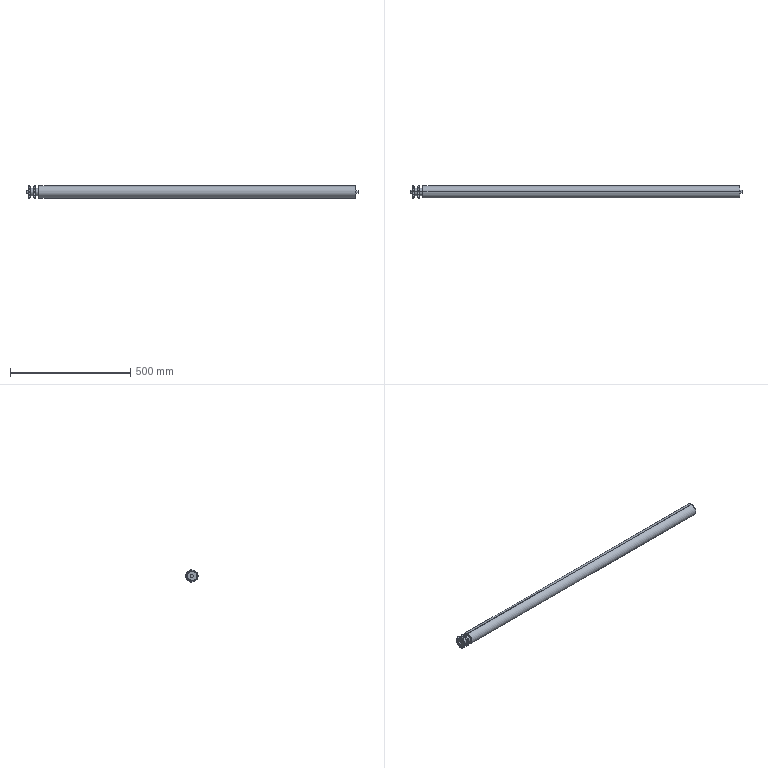Part | SolidWorks | features ICE 6, BaseBody 1, HoleWzd 1, LPattern 1 | 1 solid | 174 faces | box 1380 x 51.459 x 51.986 mm | volume 596958 mm3 | cylinder 116 | spline 44 | plane 12 | cone 2 | commonest cylinder face diameters 26.551 x46 8.595 x30 52.443 x22 12 x6 6.8 x4 32 x4